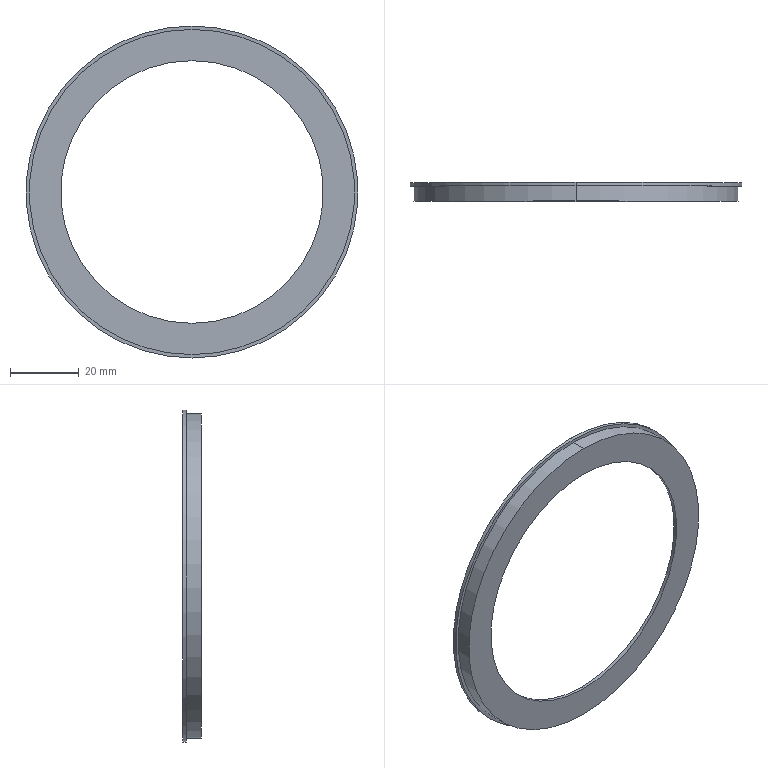Part | SolidWorks | features BaseBody 1 | 1 solid | 12 faces | box 96.7 x 5.4 x 96.7 mm | volume 4553 mm3 | cylinder 8 | plane 4 | commonest cylinder face diameters 76.5 x2 91.9 x2 94.7 x2 96.7 x2
STEP:
#1=CARTESIAN_POINT('',(-2132.95,1020.569,-1615.874));
#2=VERTEX_POINT('',#1);
#3=CARTESIAN_POINT('',(-2132.95,1020.569,-1539.374));
#4=VERTEX_POINT('',#3);
#5=CARTESIAN_POINT('',(-2132.95,1020.569,-1577.624));
#6=DIRECTION('',(0.,-1.,0.));
#7=DIRECTION('',(0.,0.,-1.));
#8=AXIS2_PLACEMENT_3D('',#5,#6,#7);
#9=CIRCLE('',#8,38.25);
#10=EDGE_CURVE('',#2,#4,#9,.T.);
#11=ORIENTED_EDGE('',*,*,#10,.F.);
#12=CARTESIAN_POINT('',(-2132.95,1020.569,-1577.624));
#13=DIRECTION('',(0.,-1.,0.));
#14=DIRECTION('',(0.,0.,1.));
#15=AXIS2_PLACEMENT_3D('',#12,#13,#14);
#16=CIRCLE('',#15,38.25);
#17=EDGE_CURVE('',#4,#2,#16,.T.);
#18=ORIENTED_EDGE('',*,*,#17,.F.);
#19=EDGE_LOOP('',(#11,#18));
#20=FACE_BOUND('',#19,.T.);
#21=CARTESIAN_POINT('',(-2132.95,1020.569,-1624.974));
#22=VERTEX_POINT('',#21);
#23=CARTESIAN_POINT('',(-2132.95,1020.569,-1530.274));
#24=VERTEX_POINT('',#23);
#25=CARTESIAN_POINT('',(-2132.95,1020.569,-1577.624));
#26=DIRECTION('',(0.,-1.,0.));
#27=DIRECTION('',(0.,0.,-1.));
#28=AXIS2_PLACEMENT_3D('',#25,#26,#27);
#29=CIRCLE('',#28,47.35);
#30=EDGE_CURVE('',#22,#24,#29,.T.);
#31=ORIENTED_EDGE('',*,*,#30,.T.);
#32=CARTESIAN_POINT('',(-2132.95,1020.569,-1577.624));
#33=DIRECTION('',(0.,-1.,0.));
#34=DIRECTION('',(0.,0.,1.));
#35=AXIS2_PLACEMENT_3D('',#32,#33,#34);
#36=CIRCLE('',#35,47.35);
#37=EDGE_CURVE('',#24,#22,#36,.T.);
#38=ORIENTED_EDGE('',*,*,#37,.T.);
#39=EDGE_LOOP('',(#31,#38));
#40=FACE_OUTER_BOUND('',#39,.T.);
#41=CARTESIAN_POINT('',(-2185.035,1020.569,-1525.539));
#42=DIRECTION('',(0.,-1.,0.));
#43=DIRECTION('',(0.,0.,-1.));
#44=AXIS2_PLACEMENT_3D('',#41,#42,#43);
#45=PLANE('',#44);
#46=ADVANCED_FACE('',(#20,#40),#45,.T.);
#47=CARTESIAN_POINT('',(-2132.95,1021.569,-1539.374));
#48=VERTEX_POINT('',#47);
#49=CARTESIAN_POINT('',(-2132.95,1020.569,-1539.374));
#50=DIRECTION('',(0.,1.,0.));
#51=VECTOR('',#50,1000.);
#52=LINE('',#49,#51);
#53=EDGE_CURVE('',#4,#48,#52,.T.);
#54=ORIENTED_EDGE('',*,*,#53,.T.);
#55=CARTESIAN_POINT('',(-2132.95,1021.569,-1615.874));
#56=VERTEX_POINT('',#55);
#57=CARTESIAN_POINT('',(-2132.95,1021.569,-1577.624));
#58=DIRECTION('',(0.,1.,0.));
#59=DIRECTION('',(0.,0.,1.));
#60=AXIS2_PLACEMENT_3D('',#57,#58,#59);
#61=CIRCLE('',#60,38.25);
#62=EDGE_CURVE('',#48,#56,#61,.T.);
#63=ORIENTED_EDGE('',*,*,#62,.T.);
#64=CARTESIAN_POINT('',(-2132.95,1021.569,-1615.874));
#65=DIRECTION('',(0.,-1.,0.));
#66=VECTOR('',#65,1000.);
#67=LINE('',#64,#66);
#68=EDGE_CURVE('',#56,#2,#67,.T.);
#69=ORIENTED_EDGE('',*,*,#68,.T.);
#70=ORIENTED_EDGE('',*,*,#10,.T.);
#71=EDGE_LOOP('',(#54,#63,#69,#70));
#72=FACE_OUTER_BOUND('',#71,.T.);
#73=CARTESIAN_POINT('',(-2132.95,1021.619,-1577.624));
#74=DIRECTION('',(0.,-1.,0.));
#75=DIRECTION('',(-0.08716,0.,-0.9962));
#76=AXIS2_PLACEMENT_3D('',#73,#74,#75);
#77=CYLINDRICAL_SURFACE('',#76,38.25);
#78=ADVANCED_FACE('',(#72),#77,.F.);
#79=ORIENTED_EDGE('',*,*,#62,.F.);
#80=CARTESIAN_POINT('',(-2132.95,1021.569,-1577.624));
#81=DIRECTION('',(0.,1.,0.));
#82=DIRECTION('',(0.,0.,-1.));
#83=AXIS2_PLACEMENT_3D('',#80,#81,#82);
#84=CIRCLE('',#83,38.25);
#85=EDGE_CURVE('',#56,#48,#84,.T.);
#86=ORIENTED_EDGE('',*,*,#85,.F.);
#87=EDGE_LOOP('',(#79,#86));
#88=FACE_BOUND('',#87,.T.);
#89=CARTESIAN_POINT('',(-2132.95,1021.569,-1531.674));
#90=VERTEX_POINT('',#89);
#91=CARTESIAN_POINT('',(-2132.95,1021.569,-1623.574));
#92=VERTEX_POINT('',#91);
#93=CARTESIAN_POINT('',(-2132.95,1021.569,-1577.624));
#94=DIRECTION('',(0.,1.,0.));
#95=DIRECTION('',(0.,0.,1.));
#96=AXIS2_PLACEMENT_3D('',#93,#94,#95);
#97=CIRCLE('',#96,45.95);
#98=EDGE_CURVE('',#90,#92,#97,.T.);
#99=ORIENTED_EDGE('',*,*,#98,.T.);
#100=CARTESIAN_POINT('',(-2132.95,1021.569,-1577.624));
#101=DIRECTION('',(0.,1.,0.));
#102=DIRECTION('',(0.,0.,-1.));
#103=AXIS2_PLACEMENT_3D('',#100,#101,#102);
#104=CIRCLE('',#103,45.95);
#105=EDGE_CURVE('',#92,#90,#104,.T.);
#106=ORIENTED_EDGE('',*,*,#105,.T.);
#107=EDGE_LOOP('',(#99,#106));
#108=FACE_OUTER_BOUND('',#107,.T.);
#109=CARTESIAN_POINT('',(-2183.495,1021.569,-1628.169));
#110=DIRECTION('',(0.,1.,0.));
#111=DIRECTION('',(1.,0.,0.));
#112=AXIS2_PLACEMENT_3D('',#109,#110,#111);
#113=PLANE('',#112);
#114=ADVANCED_FACE('',(#88,#108),#113,.T.);
#115=CARTESIAN_POINT('',(-2132.95,1025.969,-1531.674));
#116=VERTEX_POINT('',#115);
#117=CARTESIAN_POINT('',(-2132.95,1021.569,-1531.674));
#118=DIRECTION('',(0.,1.,0.));
#119=VECTOR('',#118,1000.);
#120=LINE('',#117,#119);
#121=EDGE_CURVE('',#90,#116,#120,.T.);
#122=ORIENTED_EDGE('',*,*,#121,.T.);
#123=CARTESIAN_POINT('',(-2132.95,1025.969,-1623.574));
#124=VERTEX_POINT('',#123);
#125=CARTESIAN_POINT('',(-2132.95,1025.969,-1577.624));
#126=DIRECTION('',(0.,1.,0.));
#127=DIRECTION('',(0.,0.,1.));
#128=AXIS2_PLACEMENT_3D('',#125,#126,#127);
#129=CIRCLE('',#128,45.95);
#130=EDGE_CURVE('',#116,#124,#129,.T.);
#131=ORIENTED_EDGE('',*,*,#130,.T.);
#132=CARTESIAN_POINT('',(-2132.95,1025.969,-1623.574));
#133=DIRECTION('',(0.,-1.,0.));
#134=VECTOR('',#133,1000.);
#135=LINE('',#132,#134);
#136=EDGE_CURVE('',#124,#92,#135,.T.);
#137=ORIENTED_EDGE('',*,*,#136,.T.);
#138=ORIENTED_EDGE('',*,*,#98,.F.);
#139=EDGE_LOOP('',(#122,#131,#137,#138));
#140=FACE_OUTER_BOUND('',#139,.T.);
#141=CARTESIAN_POINT('',(-2132.95,1026.189,-1577.624));
#142=DIRECTION('',(0.,-1.,0.));
#143=DIRECTION('',(-0.08716,0.,-0.9962));
#144=AXIS2_PLACEMENT_3D('',#141,#142,#143);
#145=CYLINDRICAL_SURFACE('',#144,45.95);
#146=ADVANCED_FACE('',(#140),#145,.F.);
#147=ORIENTED_EDGE('',*,*,#130,.F.);
#148=CARTESIAN_POINT('',(-2132.95,1025.969,-1577.624));
#149=DIRECTION('',(0.,1.,0.));
#150=DIRECTION('',(0.,0.,-1.));
#151=AXIS2_PLACEMENT_3D('',#148,#149,#150);
#152=CIRCLE('',#151,45.95);
#153=EDGE_CURVE('',#124,#116,#152,.T.);
#154=ORIENTED_EDGE('',*,*,#153,.F.);
#155=EDGE_LOOP('',(#147,#154));
#156=FACE_BOUND('',#155,.T.);
#157=CARTESIAN_POINT('',(-2132.95,1025.969,-1529.274));
#158=VERTEX_POINT('',#157);
#159=CARTESIAN_POINT('',(-2132.95,1025.969,-1625.974));
#160=VERTEX_POINT('',#159);
#161=CARTESIAN_POINT('',(-2132.95,1025.969,-1577.624));
#162=DIRECTION('',(0.,1.,0.));
#163=DIRECTION('',(0.,0.,1.));
#164=AXIS2_PLACEMENT_3D('',#161,#162,#163);
#165=CIRCLE('',#164,48.35);
#166=EDGE_CURVE('',#158,#160,#165,.T.);
#167=ORIENTED_EDGE('',*,*,#166,.T.);
#168=CARTESIAN_POINT('',(-2132.95,1025.969,-1577.624));
#169=DIRECTION('',(0.,1.,0.));
#170=DIRECTION('',(0.,0.,-1.));
#171=AXIS2_PLACEMENT_3D('',#168,#169,#170);
#172=CIRCLE('',#171,48.35);
#173=EDGE_CURVE('',#160,#158,#172,.T.);
#174=ORIENTED_EDGE('',*,*,#173,.T.);
#175=EDGE_LOOP('',(#167,#174));
#176=FACE_OUTER_BOUND('',#175,.T.);
#177=CARTESIAN_POINT('',(-2186.095,1025.969,-1630.809));
#178=DIRECTION('',(0.,1.,0.));
#179=DIRECTION('',(1.,0.,0.));
#180=AXIS2_PLACEMENT_3D('',#177,#178,#179);
#181=PLANE('',#180);
#182=ADVANCED_FACE('',(#156,#176),#181,.T.);
#183=CARTESIAN_POINT('',(-2132.95,1024.969,-1529.274));
#184=VERTEX_POINT('',#183);
#185=CARTESIAN_POINT('',(-2132.95,1024.969,-1529.274));
#186=DIRECTION('',(0.,1.,0.));
#187=VECTOR('',#186,1000.);
#188=LINE('',#185,#187);
#189=EDGE_CURVE('',#184,#158,#188,.T.);
#190=ORIENTED_EDGE('',*,*,#189,.T.);
#191=ORIENTED_EDGE('',*,*,#173,.F.);
#192=CARTESIAN_POINT('',(-2132.95,1024.969,-1625.974));
#193=VERTEX_POINT('',#192);
#194=CARTESIAN_POINT('',(-2132.95,1025.969,-1625.974));
#195=DIRECTION('',(0.,-1.,0.));
#196=VECTOR('',#195,1000.);
#197=LINE('',#194,#196);
#198=EDGE_CURVE('',#160,#193,#197,.T.);
#199=ORIENTED_EDGE('',*,*,#198,.T.);
#200=CARTESIAN_POINT('',(-2132.95,1024.969,-1577.624));
#201=DIRECTION('',(0.,-1.,0.));
#202=DIRECTION('',(0.,0.,1.));
#203=AXIS2_PLACEMENT_3D('',#200,#201,#202);
#204=CIRCLE('',#203,48.35);
#205=EDGE_CURVE('',#184,#193,#204,.T.);
#206=ORIENTED_EDGE('',*,*,#205,.F.);
#207=EDGE_LOOP('',(#190,#191,#199,#206));
#208=FACE_OUTER_BOUND('',#207,.T.);
#209=CARTESIAN_POINT('',(-2132.95,1024.919,-1577.624));
#210=DIRECTION('',(0.,-1.,0.));
#211=DIRECTION('',(0.08716,0.,0.9962));
#212=AXIS2_PLACEMENT_3D('',#209,#210,#211);
#213=CYLINDRICAL_SURFACE('',#212,48.35);
#214=ADVANCED_FACE('',(#208),#213,.T.);
#215=CARTESIAN_POINT('',(-2132.95,1024.969,-1624.974));
#216=VERTEX_POINT('',#215);
#217=CARTESIAN_POINT('',(-2132.95,1024.969,-1530.274));
#218=VERTEX_POINT('',#217);
#219=CARTESIAN_POINT('',(-2132.95,1024.969,-1577.624));
#220=DIRECTION('',(0.,-1.,0.));
#221=DIRECTION('',(0.,0.,-1.));
#222=AXIS2_PLACEMENT_3D('',#219,#220,#221);
#223=CIRCLE('',#222,47.35);
#224=EDGE_CURVE('',#216,#218,#223,.T.);
#225=ORIENTED_EDGE('',*,*,#224,.F.);
#226=CARTESIAN_POINT('',(-2132.95,1024.969,-1577.624));
#227=DIRECTION('',(0.,-1.,0.));
#228=DIRECTION('',(0.,0.,1.));
#229=AXIS2_PLACEMENT_3D('',#226,#227,#228);
#230=CIRCLE('',#229,47.35);
#231=EDGE_CURVE('',#218,#216,#230,.T.);
#232=ORIENTED_EDGE('',*,*,#231,.F.);
#233=EDGE_LOOP('',(#225,#232));
#234=FACE_BOUND('',#233,.T.);
#235=CARTESIAN_POINT('',(-2132.95,1024.969,-1577.624));
#236=DIRECTION('',(0.,-1.,0.));
#237=DIRECTION('',(0.,0.,-1.));
#238=AXIS2_PLACEMENT_3D('',#235,#236,#237);
#239=CIRCLE('',#238,48.35);
#240=EDGE_CURVE('',#193,#184,#239,.T.);
#241=ORIENTED_EDGE('',*,*,#240,.T.);
#242=ORIENTED_EDGE('',*,*,#205,.T.);
#243=EDGE_LOOP('',(#241,#242));
#244=FACE_OUTER_BOUND('',#243,.T.);
#245=CARTESIAN_POINT('',(-2186.095,1024.969,-1524.439));
#246=DIRECTION('',(0.,-1.,0.));
#247=DIRECTION('',(0.,0.,-1.));
#248=AXIS2_PLACEMENT_3D('',#245,#246,#247);
#249=PLANE('',#248);
#250=ADVANCED_FACE('',(#234,#244),#249,.T.);
#251=CARTESIAN_POINT('',(-2132.95,1020.569,-1530.274));
#252=DIRECTION('',(0.,1.,0.));
#253=VECTOR('',#252,1000.);
#254=LINE('',#251,#253);
#255=EDGE_CURVE('',#24,#218,#254,.T.);
#256=ORIENTED_EDGE('',*,*,#255,.T.);
#257=ORIENTED_EDGE('',*,*,#231,.T.);
#258=CARTESIAN_POINT('',(-2132.95,1024.969,-1624.974));
#259=DIRECTION('',(0.,-1.,0.));
#260=VECTOR('',#259,1000.);
#261=LINE('',#258,#260);
#262=EDGE_CURVE('',#216,#22,#261,.T.);
#263=ORIENTED_EDGE('',*,*,#262,.T.);
#264=ORIENTED_EDGE('',*,*,#37,.F.);
#265=EDGE_LOOP('',(#256,#257,#263,#264));
#266=FACE_OUTER_BOUND('',#265,.T.);
#267=CARTESIAN_POINT('',(-2132.95,1020.349,-1577.624));
#268=DIRECTION('',(0.,-1.,0.));
#269=DIRECTION('',(0.08716,0.,0.9962));
#270=AXIS2_PLACEMENT_3D('',#267,#268,#269);
#271=CYLINDRICAL_SURFACE('',#270,47.35);
#272=ADVANCED_FACE('',(#266),#271,.T.);
#273=ORIENTED_EDGE('',*,*,#255,.F.);
#274=ORIENTED_EDGE('',*,*,#30,.F.);
#275=ORIENTED_EDGE('',*,*,#262,.F.);
#276=ORIENTED_EDGE('',*,*,#224,.T.);
#277=EDGE_LOOP('',(#273,#274,#275,#276));
#278=FACE_OUTER_BOUND('',#277,.T.);
#279=CARTESIAN_POINT('',(-2132.95,1020.349,-1577.624));
#280=DIRECTION('',(0.,-1.,0.));
#281=DIRECTION('',(-0.08716,0.,-0.9962));
#282=AXIS2_PLACEMENT_3D('',#279,#280,#281);
#283=CYLINDRICAL_SURFACE('',#282,47.35);
#284=ADVANCED_FACE('',(#278),#283,.T.);
#285=ORIENTED_EDGE('',*,*,#189,.F.);
#286=ORIENTED_EDGE('',*,*,#240,.F.);
#287=ORIENTED_EDGE('',*,*,#198,.F.);
#288=ORIENTED_EDGE('',*,*,#166,.F.);
#289=EDGE_LOOP('',(#285,#286,#287,#288));
#290=FACE_OUTER_BOUND('',#289,.T.);
#291=CARTESIAN_POINT('',(-2132.95,1024.919,-1577.624));
#292=DIRECTION('',(0.,-1.,0.));
#293=DIRECTION('',(-0.08716,0.,-0.9962));
#294=AXIS2_PLACEMENT_3D('',#291,#292,#293);
#295=CYLINDRICAL_SURFACE('',#294,48.35);
#296=ADVANCED_FACE('',(#290),#295,.T.);
#297=ORIENTED_EDGE('',*,*,#121,.F.);
#298=ORIENTED_EDGE('',*,*,#105,.F.);
#299=ORIENTED_EDGE('',*,*,#136,.F.);
#300=ORIENTED_EDGE('',*,*,#153,.T.);
#301=EDGE_LOOP('',(#297,#298,#299,#300));
#302=FACE_OUTER_BOUND('',#301,.T.);
#303=CARTESIAN_POINT('',(-2132.95,1026.189,-1577.624));
#304=DIRECTION('',(0.,-1.,0.));
#305=DIRECTION('',(0.08716,0.,0.9962));
#306=AXIS2_PLACEMENT_3D('',#303,#304,#305);
#307=CYLINDRICAL_SURFACE('',#306,45.95);
#308=ADVANCED_FACE('',(#302),#307,.F.);
#309=ORIENTED_EDGE('',*,*,#53,.F.);
#310=ORIENTED_EDGE('',*,*,#17,.T.);
#311=ORIENTED_EDGE('',*,*,#68,.F.);
#312=ORIENTED_EDGE('',*,*,#85,.T.);
#313=EDGE_LOOP('',(#309,#310,#311,#312));
#314=FACE_OUTER_BOUND('',#313,.T.);
#315=CARTESIAN_POINT('',(-2132.95,1021.619,-1577.624));
#316=DIRECTION('',(0.,-1.,0.));
#317=DIRECTION('',(0.08716,0.,0.9962));
#318=AXIS2_PLACEMENT_3D('',#315,#316,#317);
#319=CYLINDRICAL_SURFACE('',#318,38.25);
#320=ADVANCED_FACE('',(#314),#319,.F.);
#321=CLOSED_SHELL('',(#46,#78,#114,#146,#182,#214,#250,#272,#284,#296,#308,#320));
#322=MANIFOLD_SOLID_BREP('',#321);
#323=CARTESIAN_POINT('',(0.,0.,0.));
#324=DIRECTION('',(0.,0.,1.));
#325=DIRECTION('',(1.,0.,0.));
#326=AXIS2_PLACEMENT_3D('',#323,#324,#325);
#327=(LENGTH_UNIT()NAMED_UNIT(*)SI_UNIT(.MILLI.,.METRE.));
#328=UNCERTAINTY_MEASURE_WITH_UNIT(LENGTH_MEASURE(0.00001),#327,'','');
#329=(NAMED_UNIT(*)PLANE_ANGLE_UNIT()SI_UNIT($,.RADIAN.));
#330=(NAMED_UNIT(*)SI_UNIT($,.STERADIAN.)SOLID_ANGLE_UNIT());
#331=(GEOMETRIC_REPRESENTATION_CONTEXT(3)GLOBAL_UNCERTAINTY_ASSIGNED_CONTEXT((#328))GLOBAL_UNIT_ASSIGNED_CONTEXT((#327,#329,#330))REPRESENTATION_CONTEXT('',''));
#332=ADVANCED_BREP_SHAPE_REPRESENTATION('',(#322,#326),#331);